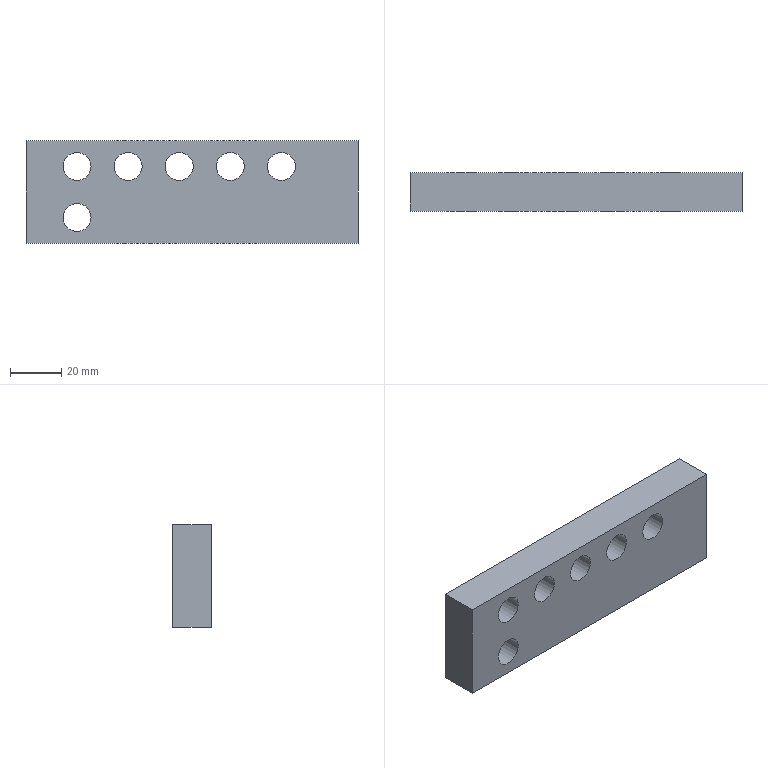Part | NX | features DATUM_CSYS 2, EXTRUDE 1, SKETCH 1 | 1 solid | 12 faces | box 130 x 15 x 40 mm | volume 69447 mm3 | plane 6 | cylinder 6 | commonest cylinder face diameters 11 x6
STEP:
#1=CARTESIAN_POINT('',(-65.,0.,20.));
#2=VERTEX_POINT('',#1);
#3=CARTESIAN_POINT('',(-65.,0.,-20.));
#4=VERTEX_POINT('',#3);
#5=CARTESIAN_POINT('',(-65.,0.,20.));
#6=DIRECTION('',(0.,0.,-1.));
#7=VECTOR('',#6,1000.);
#8=LINE('',#5,#7);
#9=EDGE_CURVE('',#2,#4,#8,.T.);
#10=ORIENTED_EDGE('',*,*,#9,.T.);
#11=CARTESIAN_POINT('',(-65.,-15.,-20.));
#12=VERTEX_POINT('',#11);
#13=CARTESIAN_POINT('',(-65.,-15.,-20.));
#14=DIRECTION('',(0.,1.,0.));
#15=VECTOR('',#14,1000.);
#16=LINE('',#13,#15);
#17=EDGE_CURVE('',#12,#4,#16,.T.);
#18=ORIENTED_EDGE('',*,*,#17,.F.);
#19=CARTESIAN_POINT('',(-65.,-15.,20.));
#20=VERTEX_POINT('',#19);
#21=CARTESIAN_POINT('',(-65.,-15.,20.));
#22=DIRECTION('',(0.,0.,-1.));
#23=VECTOR('',#22,1000.);
#24=LINE('',#21,#23);
#25=EDGE_CURVE('',#20,#12,#24,.T.);
#26=ORIENTED_EDGE('',*,*,#25,.F.);
#27=CARTESIAN_POINT('',(-65.,-15.,20.));
#28=DIRECTION('',(0.,1.,0.));
#29=VECTOR('',#28,1000.);
#30=LINE('',#27,#29);
#31=EDGE_CURVE('',#20,#2,#30,.T.);
#32=ORIENTED_EDGE('',*,*,#31,.T.);
#33=EDGE_LOOP('',(#10,#18,#26,#32));
#34=FACE_BOUND('',#33,.T.);
#35=CARTESIAN_POINT('',(-65.,-15.,20.));
#36=DIRECTION('',(1.,0.,0.));
#37=DIRECTION('',(0.,0.,-1.));
#38=AXIS2_PLACEMENT_3D('',#35,#36,#37);
#39=PLANE('',#38);
#40=ADVANCED_FACE('',(#34),#39,.F.);
#41=CARTESIAN_POINT('',(65.,0.,-20.));
#42=VERTEX_POINT('',#41);
#43=CARTESIAN_POINT('',(-65.,0.,-20.));
#44=DIRECTION('',(1.,0.,0.));
#45=VECTOR('',#44,1000.);
#46=LINE('',#43,#45);
#47=EDGE_CURVE('',#4,#42,#46,.T.);
#48=ORIENTED_EDGE('',*,*,#47,.T.);
#49=CARTESIAN_POINT('',(65.,-15.,-20.));
#50=VERTEX_POINT('',#49);
#51=CARTESIAN_POINT('',(65.,-15.,-20.));
#52=DIRECTION('',(0.,1.,0.));
#53=VECTOR('',#52,1000.);
#54=LINE('',#51,#53);
#55=EDGE_CURVE('',#50,#42,#54,.T.);
#56=ORIENTED_EDGE('',*,*,#55,.F.);
#57=CARTESIAN_POINT('',(-65.,-15.,-20.));
#58=DIRECTION('',(1.,0.,0.));
#59=VECTOR('',#58,1000.);
#60=LINE('',#57,#59);
#61=EDGE_CURVE('',#12,#50,#60,.T.);
#62=ORIENTED_EDGE('',*,*,#61,.F.);
#63=ORIENTED_EDGE('',*,*,#17,.T.);
#64=EDGE_LOOP('',(#48,#56,#62,#63));
#65=FACE_BOUND('',#64,.T.);
#66=CARTESIAN_POINT('',(-65.,-15.,-20.));
#67=DIRECTION('',(0.,0.,1.));
#68=DIRECTION('',(1.,0.,0.));
#69=AXIS2_PLACEMENT_3D('',#66,#67,#68);
#70=PLANE('',#69);
#71=ADVANCED_FACE('',(#65),#70,.F.);
#72=CARTESIAN_POINT('',(65.,0.,20.));
#73=VERTEX_POINT('',#72);
#74=CARTESIAN_POINT('',(65.,0.,-20.));
#75=DIRECTION('',(0.,0.,1.));
#76=VECTOR('',#75,1000.);
#77=LINE('',#74,#76);
#78=EDGE_CURVE('',#42,#73,#77,.T.);
#79=ORIENTED_EDGE('',*,*,#78,.T.);
#80=CARTESIAN_POINT('',(65.,-15.,20.));
#81=VERTEX_POINT('',#80);
#82=CARTESIAN_POINT('',(65.,-15.,20.));
#83=DIRECTION('',(0.,1.,0.));
#84=VECTOR('',#83,1000.);
#85=LINE('',#82,#84);
#86=EDGE_CURVE('',#81,#73,#85,.T.);
#87=ORIENTED_EDGE('',*,*,#86,.F.);
#88=CARTESIAN_POINT('',(65.,-15.,-20.));
#89=DIRECTION('',(0.,0.,1.));
#90=VECTOR('',#89,1000.);
#91=LINE('',#88,#90);
#92=EDGE_CURVE('',#50,#81,#91,.T.);
#93=ORIENTED_EDGE('',*,*,#92,.F.);
#94=ORIENTED_EDGE('',*,*,#55,.T.);
#95=EDGE_LOOP('',(#79,#87,#93,#94));
#96=FACE_BOUND('',#95,.T.);
#97=CARTESIAN_POINT('',(65.,-15.,-20.));
#98=DIRECTION('',(-1.,0.,0.));
#99=DIRECTION('',(0.,0.,1.));
#100=AXIS2_PLACEMENT_3D('',#97,#98,#99);
#101=PLANE('',#100);
#102=ADVANCED_FACE('',(#96),#101,.F.);
#103=CARTESIAN_POINT('',(0.5,-15.,10.));
#104=VERTEX_POINT('',#103);
#105=CARTESIAN_POINT('',(-5.,-15.,10.));
#106=DIRECTION('',(0.,-1.,0.));
#107=DIRECTION('',(1.,0.,0.));
#108=AXIS2_PLACEMENT_3D('',#105,#106,#107);
#109=CIRCLE('',#108,5.5);
#110=EDGE_CURVE('',#104,#104,#109,.T.);
#111=ORIENTED_EDGE('',*,*,#110,.T.);
#112=EDGE_LOOP('',(#111));
#113=FACE_BOUND('',#112,.T.);
#114=CARTESIAN_POINT('',(0.5,0.,10.));
#115=VERTEX_POINT('',#114);
#116=CARTESIAN_POINT('',(-5.,0.,10.));
#117=DIRECTION('',(0.,-1.,0.));
#118=DIRECTION('',(1.,0.,0.));
#119=AXIS2_PLACEMENT_3D('',#116,#117,#118);
#120=CIRCLE('',#119,5.5);
#121=EDGE_CURVE('',#115,#115,#120,.T.);
#122=ORIENTED_EDGE('',*,*,#121,.F.);
#123=EDGE_LOOP('',(#122));
#124=FACE_BOUND('',#123,.T.);
#125=CARTESIAN_POINT('',(-5.,-15.,10.));
#126=DIRECTION('',(0.,1.,0.));
#127=DIRECTION('',(0.,0.,1.));
#128=AXIS2_PLACEMENT_3D('',#125,#126,#127);
#129=CYLINDRICAL_SURFACE('',#128,5.5);
#130=ADVANCED_FACE('',(#113,#124),#129,.F.);
#131=CARTESIAN_POINT('',(-39.5,-15.,10.));
#132=VERTEX_POINT('',#131);
#133=CARTESIAN_POINT('',(-45.,-15.,10.));
#134=DIRECTION('',(0.,-1.,0.));
#135=DIRECTION('',(1.,0.,0.));
#136=AXIS2_PLACEMENT_3D('',#133,#134,#135);
#137=CIRCLE('',#136,5.5);
#138=EDGE_CURVE('',#132,#132,#137,.T.);
#139=ORIENTED_EDGE('',*,*,#138,.T.);
#140=EDGE_LOOP('',(#139));
#141=FACE_BOUND('',#140,.T.);
#142=CARTESIAN_POINT('',(-39.5,0.,10.));
#143=VERTEX_POINT('',#142);
#144=CARTESIAN_POINT('',(-45.,0.,10.));
#145=DIRECTION('',(0.,-1.,0.));
#146=DIRECTION('',(1.,0.,0.));
#147=AXIS2_PLACEMENT_3D('',#144,#145,#146);
#148=CIRCLE('',#147,5.5);
#149=EDGE_CURVE('',#143,#143,#148,.T.);
#150=ORIENTED_EDGE('',*,*,#149,.F.);
#151=EDGE_LOOP('',(#150));
#152=FACE_BOUND('',#151,.T.);
#153=CARTESIAN_POINT('',(-45.,-15.,10.));
#154=DIRECTION('',(0.,1.,0.));
#155=DIRECTION('',(0.,0.,1.));
#156=AXIS2_PLACEMENT_3D('',#153,#154,#155);
#157=CYLINDRICAL_SURFACE('',#156,5.5);
#158=ADVANCED_FACE('',(#141,#152),#157,.F.);
#159=CARTESIAN_POINT('',(-39.5,-15.,-10.));
#160=VERTEX_POINT('',#159);
#161=CARTESIAN_POINT('',(-45.,-15.,-10.));
#162=DIRECTION('',(0.,-1.,0.));
#163=DIRECTION('',(1.,0.,0.));
#164=AXIS2_PLACEMENT_3D('',#161,#162,#163);
#165=CIRCLE('',#164,5.5);
#166=EDGE_CURVE('',#160,#160,#165,.T.);
#167=ORIENTED_EDGE('',*,*,#166,.T.);
#168=EDGE_LOOP('',(#167));
#169=FACE_BOUND('',#168,.T.);
#170=CARTESIAN_POINT('',(-39.5,0.,-10.));
#171=VERTEX_POINT('',#170);
#172=CARTESIAN_POINT('',(-45.,0.,-10.));
#173=DIRECTION('',(0.,-1.,0.));
#174=DIRECTION('',(1.,0.,0.));
#175=AXIS2_PLACEMENT_3D('',#172,#173,#174);
#176=CIRCLE('',#175,5.5);
#177=EDGE_CURVE('',#171,#171,#176,.T.);
#178=ORIENTED_EDGE('',*,*,#177,.F.);
#179=EDGE_LOOP('',(#178));
#180=FACE_BOUND('',#179,.T.);
#181=CARTESIAN_POINT('',(-45.,-15.,-10.));
#182=DIRECTION('',(0.,1.,0.));
#183=DIRECTION('',(0.,0.,1.));
#184=AXIS2_PLACEMENT_3D('',#181,#182,#183);
#185=CYLINDRICAL_SURFACE('',#184,5.5);
#186=ADVANCED_FACE('',(#169,#180),#185,.F.);
#187=CARTESIAN_POINT('',(-19.5,-15.,10.));
#188=VERTEX_POINT('',#187);
#189=CARTESIAN_POINT('',(-25.,-15.,10.));
#190=DIRECTION('',(0.,-1.,0.));
#191=DIRECTION('',(1.,0.,0.));
#192=AXIS2_PLACEMENT_3D('',#189,#190,#191);
#193=CIRCLE('',#192,5.5);
#194=EDGE_CURVE('',#188,#188,#193,.T.);
#195=ORIENTED_EDGE('',*,*,#194,.T.);
#196=EDGE_LOOP('',(#195));
#197=FACE_BOUND('',#196,.T.);
#198=CARTESIAN_POINT('',(-19.5,0.,10.));
#199=VERTEX_POINT('',#198);
#200=CARTESIAN_POINT('',(-25.,0.,10.));
#201=DIRECTION('',(0.,-1.,0.));
#202=DIRECTION('',(1.,0.,0.));
#203=AXIS2_PLACEMENT_3D('',#200,#201,#202);
#204=CIRCLE('',#203,5.5);
#205=EDGE_CURVE('',#199,#199,#204,.T.);
#206=ORIENTED_EDGE('',*,*,#205,.F.);
#207=EDGE_LOOP('',(#206));
#208=FACE_BOUND('',#207,.T.);
#209=CARTESIAN_POINT('',(-25.,-15.,10.));
#210=DIRECTION('',(0.,1.,0.));
#211=DIRECTION('',(0.,0.,1.));
#212=AXIS2_PLACEMENT_3D('',#209,#210,#211);
#213=CYLINDRICAL_SURFACE('',#212,5.5);
#214=ADVANCED_FACE('',(#197,#208),#213,.F.);
#215=CARTESIAN_POINT('',(20.5,-15.,10.));
#216=VERTEX_POINT('',#215);
#217=CARTESIAN_POINT('',(15.,-15.,10.));
#218=DIRECTION('',(0.,-1.,0.));
#219=DIRECTION('',(1.,0.,0.));
#220=AXIS2_PLACEMENT_3D('',#217,#218,#219);
#221=CIRCLE('',#220,5.5);
#222=EDGE_CURVE('',#216,#216,#221,.T.);
#223=ORIENTED_EDGE('',*,*,#222,.T.);
#224=EDGE_LOOP('',(#223));
#225=FACE_BOUND('',#224,.T.);
#226=CARTESIAN_POINT('',(20.5,0.,10.));
#227=VERTEX_POINT('',#226);
#228=CARTESIAN_POINT('',(15.,0.,10.));
#229=DIRECTION('',(0.,-1.,0.));
#230=DIRECTION('',(1.,0.,0.));
#231=AXIS2_PLACEMENT_3D('',#228,#229,#230);
#232=CIRCLE('',#231,5.5);
#233=EDGE_CURVE('',#227,#227,#232,.T.);
#234=ORIENTED_EDGE('',*,*,#233,.F.);
#235=EDGE_LOOP('',(#234));
#236=FACE_BOUND('',#235,.T.);
#237=CARTESIAN_POINT('',(15.,-15.,10.));
#238=DIRECTION('',(0.,1.,0.));
#239=DIRECTION('',(0.,0.,1.));
#240=AXIS2_PLACEMENT_3D('',#237,#238,#239);
#241=CYLINDRICAL_SURFACE('',#240,5.5);
#242=ADVANCED_FACE('',(#225,#236),#241,.F.);
#243=CARTESIAN_POINT('',(65.,0.,20.));
#244=DIRECTION('',(-1.,0.,0.));
#245=VECTOR('',#244,1000.);
#246=LINE('',#243,#245);
#247=EDGE_CURVE('',#73,#2,#246,.T.);
#248=ORIENTED_EDGE('',*,*,#247,.T.);
#249=ORIENTED_EDGE('',*,*,#31,.F.);
#250=CARTESIAN_POINT('',(65.,-15.,20.));
#251=DIRECTION('',(-1.,0.,0.));
#252=VECTOR('',#251,1000.);
#253=LINE('',#250,#252);
#254=EDGE_CURVE('',#81,#20,#253,.T.);
#255=ORIENTED_EDGE('',*,*,#254,.F.);
#256=ORIENTED_EDGE('',*,*,#86,.T.);
#257=EDGE_LOOP('',(#248,#249,#255,#256));
#258=FACE_BOUND('',#257,.T.);
#259=CARTESIAN_POINT('',(65.,-15.,20.));
#260=DIRECTION('',(0.,0.,-1.));
#261=DIRECTION('',(-1.,0.,0.));
#262=AXIS2_PLACEMENT_3D('',#259,#260,#261);
#263=PLANE('',#262);
#264=ADVANCED_FACE('',(#258),#263,.F.);
#265=CARTESIAN_POINT('',(40.5,-15.,10.));
#266=VERTEX_POINT('',#265);
#267=CARTESIAN_POINT('',(35.,-15.,10.));
#268=DIRECTION('',(0.,-1.,0.));
#269=DIRECTION('',(1.,0.,0.));
#270=AXIS2_PLACEMENT_3D('',#267,#268,#269);
#271=CIRCLE('',#270,5.5);
#272=EDGE_CURVE('',#266,#266,#271,.T.);
#273=ORIENTED_EDGE('',*,*,#272,.T.);
#274=EDGE_LOOP('',(#273));
#275=FACE_BOUND('',#274,.T.);
#276=CARTESIAN_POINT('',(40.5,0.,10.));
#277=VERTEX_POINT('',#276);
#278=CARTESIAN_POINT('',(35.,0.,10.));
#279=DIRECTION('',(0.,-1.,0.));
#280=DIRECTION('',(1.,0.,0.));
#281=AXIS2_PLACEMENT_3D('',#278,#279,#280);
#282=CIRCLE('',#281,5.5);
#283=EDGE_CURVE('',#277,#277,#282,.T.);
#284=ORIENTED_EDGE('',*,*,#283,.F.);
#285=EDGE_LOOP('',(#284));
#286=FACE_BOUND('',#285,.T.);
#287=CARTESIAN_POINT('',(35.,-15.,10.));
#288=DIRECTION('',(0.,1.,0.));
#289=DIRECTION('',(0.,0.,1.));
#290=AXIS2_PLACEMENT_3D('',#287,#288,#289);
#291=CYLINDRICAL_SURFACE('',#290,5.5);
#292=ADVANCED_FACE('',(#275,#286),#291,.F.);
#293=ORIENTED_EDGE('',*,*,#25,.T.);
#294=ORIENTED_EDGE('',*,*,#61,.T.);
#295=ORIENTED_EDGE('',*,*,#92,.T.);
#296=ORIENTED_EDGE('',*,*,#254,.T.);
#297=EDGE_LOOP('',(#293,#294,#295,#296));
#298=FACE_BOUND('',#297,.T.);
#299=ORIENTED_EDGE('',*,*,#222,.F.);
#300=EDGE_LOOP('',(#299));
#301=FACE_BOUND('',#300,.T.);
#302=ORIENTED_EDGE('',*,*,#194,.F.);
#303=EDGE_LOOP('',(#302));
#304=FACE_BOUND('',#303,.T.);
#305=ORIENTED_EDGE('',*,*,#166,.F.);
#306=EDGE_LOOP('',(#305));
#307=FACE_BOUND('',#306,.T.);
#308=ORIENTED_EDGE('',*,*,#138,.F.);
#309=EDGE_LOOP('',(#308));
#310=FACE_BOUND('',#309,.T.);
#311=ORIENTED_EDGE('',*,*,#110,.F.);
#312=EDGE_LOOP('',(#311));
#313=FACE_BOUND('',#312,.T.);
#314=ORIENTED_EDGE('',*,*,#272,.F.);
#315=EDGE_LOOP('',(#314));
#316=FACE_BOUND('',#315,.T.);
#317=CARTESIAN_POINT('',(15.,-15.,10.));
#318=DIRECTION('',(0.,-1.,0.));
#319=DIRECTION('',(0.,0.,-1.));
#320=AXIS2_PLACEMENT_3D('',#317,#318,#319);
#321=PLANE('',#320);
#322=ADVANCED_FACE('',(#298,#301,#304,#307,#310,#313,#316),#321,.T.);
#323=ORIENTED_EDGE('',*,*,#9,.F.);
#324=ORIENTED_EDGE('',*,*,#247,.F.);
#325=ORIENTED_EDGE('',*,*,#78,.F.);
#326=ORIENTED_EDGE('',*,*,#47,.F.);
#327=EDGE_LOOP('',(#323,#324,#325,#326));
#328=FACE_BOUND('',#327,.T.);
#329=ORIENTED_EDGE('',*,*,#233,.T.);
#330=EDGE_LOOP('',(#329));
#331=FACE_BOUND('',#330,.T.);
#332=ORIENTED_EDGE('',*,*,#205,.T.);
#333=EDGE_LOOP('',(#332));
#334=FACE_BOUND('',#333,.T.);
#335=ORIENTED_EDGE('',*,*,#177,.T.);
#336=EDGE_LOOP('',(#335));
#337=FACE_BOUND('',#336,.T.);
#338=ORIENTED_EDGE('',*,*,#149,.T.);
#339=EDGE_LOOP('',(#338));
#340=FACE_BOUND('',#339,.T.);
#341=ORIENTED_EDGE('',*,*,#121,.T.);
#342=EDGE_LOOP('',(#341));
#343=FACE_BOUND('',#342,.T.);
#344=ORIENTED_EDGE('',*,*,#283,.T.);
#345=EDGE_LOOP('',(#344));
#346=FACE_BOUND('',#345,.T.);
#347=CARTESIAN_POINT('',(15.,0.,10.));
#348=DIRECTION('',(0.,-1.,0.));
#349=DIRECTION('',(0.,0.,-1.));
#350=AXIS2_PLACEMENT_3D('',#347,#348,#349);
#351=PLANE('',#350);
#352=ADVANCED_FACE('',(#328,#331,#334,#337,#340,#343,#346),#351,.F.);
#353=CLOSED_SHELL('',(#40,#71,#102,#130,#158,#186,#214,#242,#264,#292,#322,#352));
#354=MANIFOLD_SOLID_BREP('',#353);
#355=(LENGTH_UNIT()NAMED_UNIT(*)SI_UNIT(.MILLI.,.METRE.));
#356=UNCERTAINTY_MEASURE_WITH_UNIT(LENGTH_MEASURE(0.00001),#355,'','');
#357=(NAMED_UNIT(*)PLANE_ANGLE_UNIT()SI_UNIT($,.RADIAN.));
#358=(NAMED_UNIT(*)SI_UNIT($,.STERADIAN.)SOLID_ANGLE_UNIT());
#359=(GEOMETRIC_REPRESENTATION_CONTEXT(3)GLOBAL_UNCERTAINTY_ASSIGNED_CONTEXT((#356))GLOBAL_UNIT_ASSIGNED_CONTEXT((#355,#357,#358))REPRESENTATION_CONTEXT('',''));
#360=ADVANCED_BREP_SHAPE_REPRESENTATION('',(#354),#359);